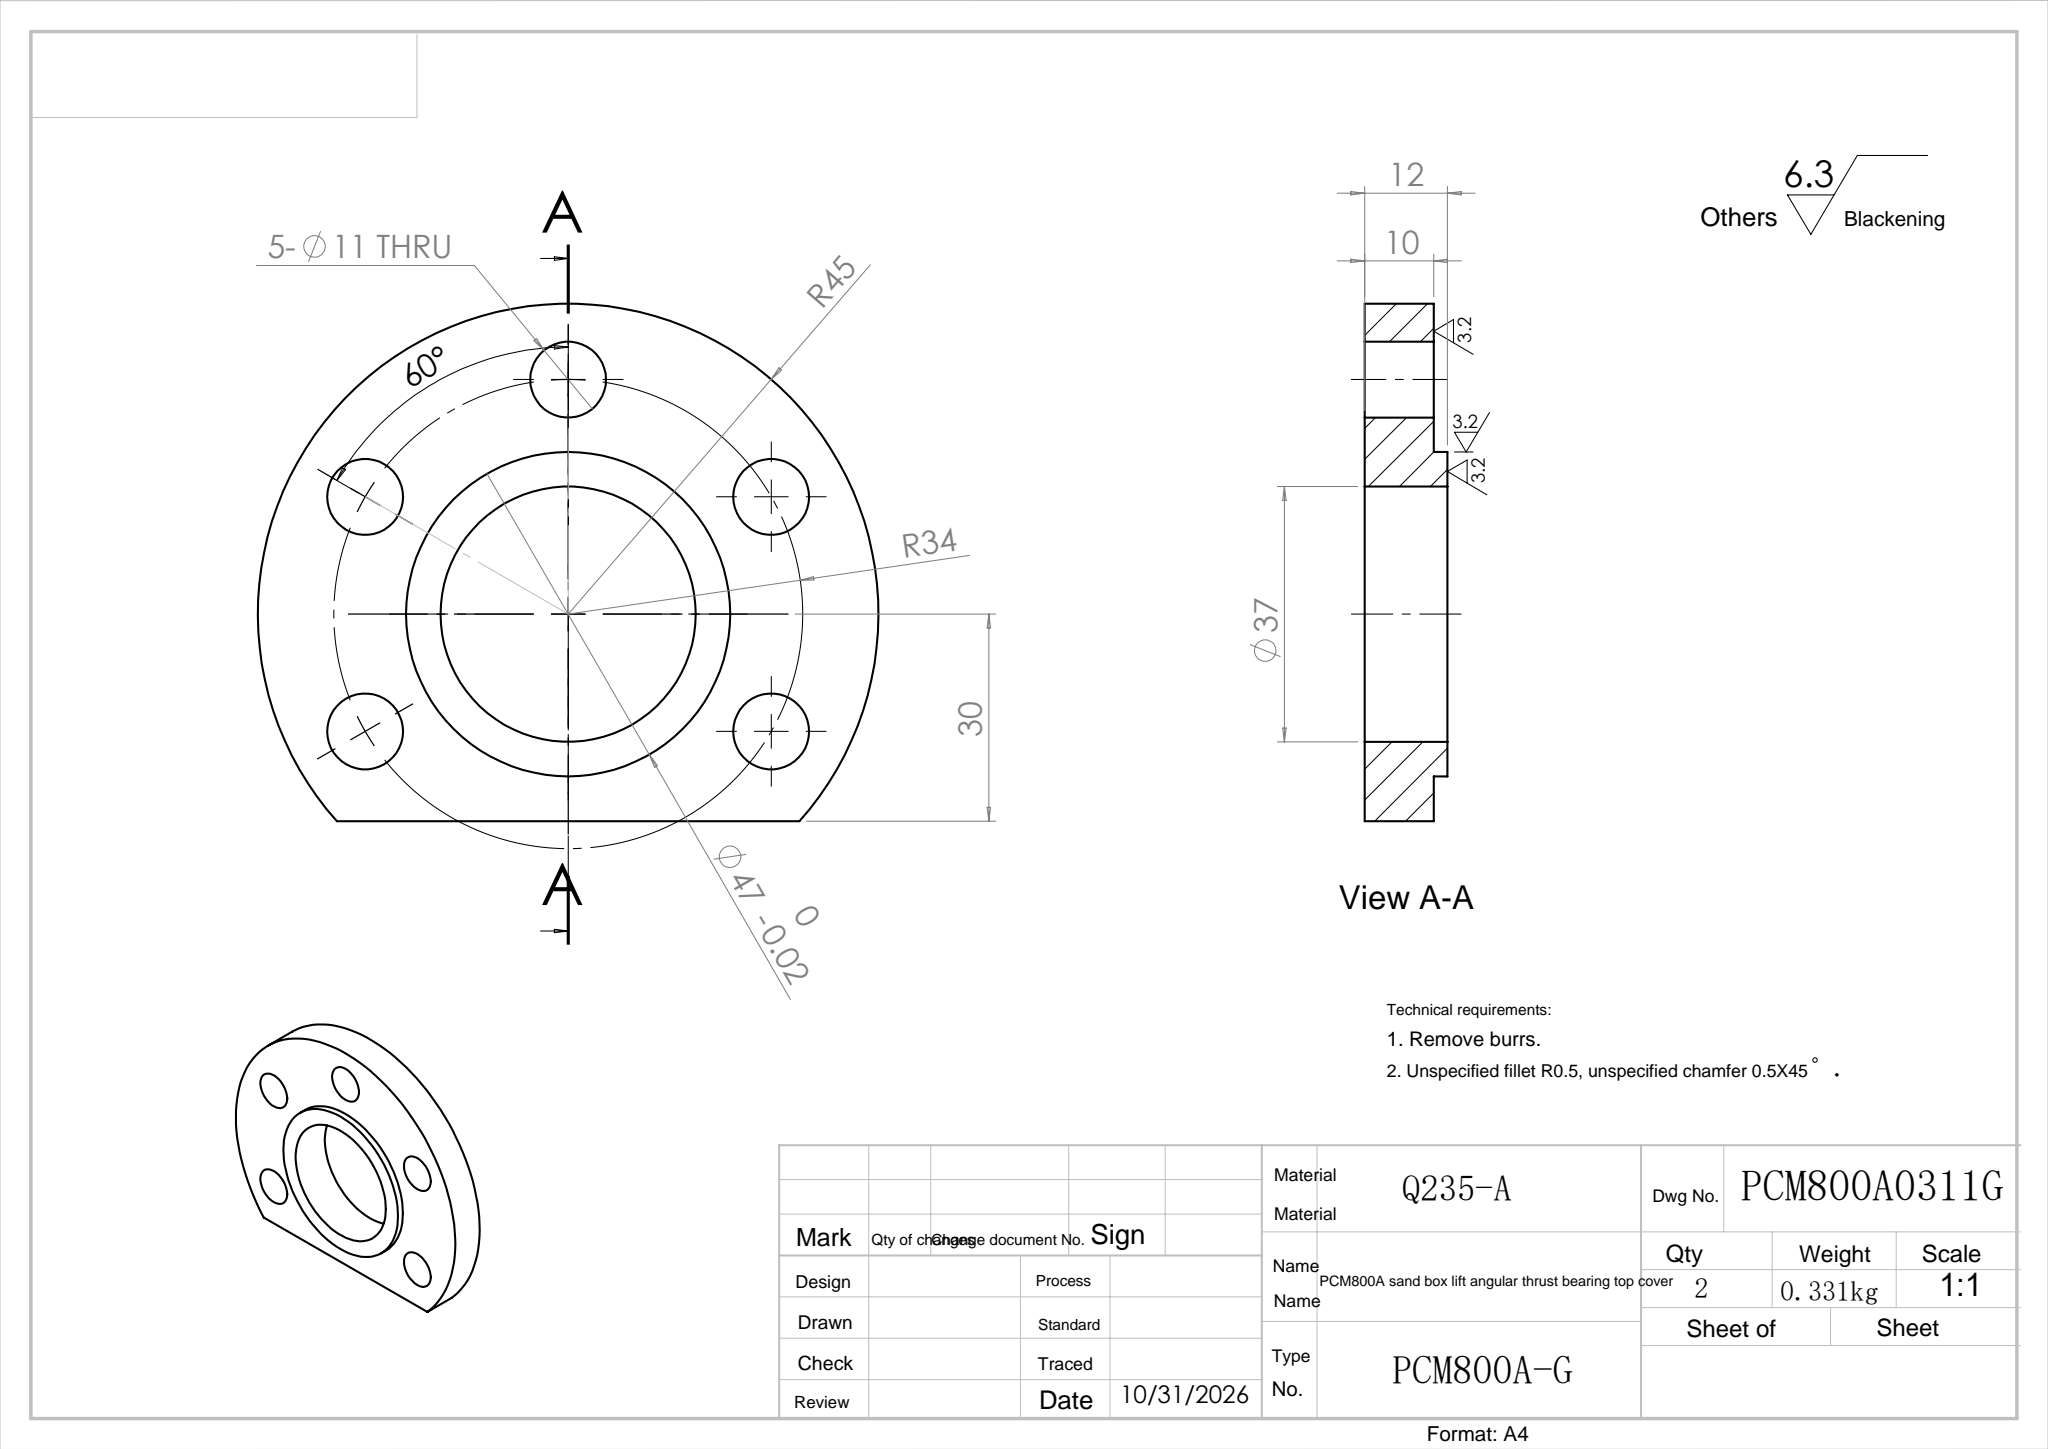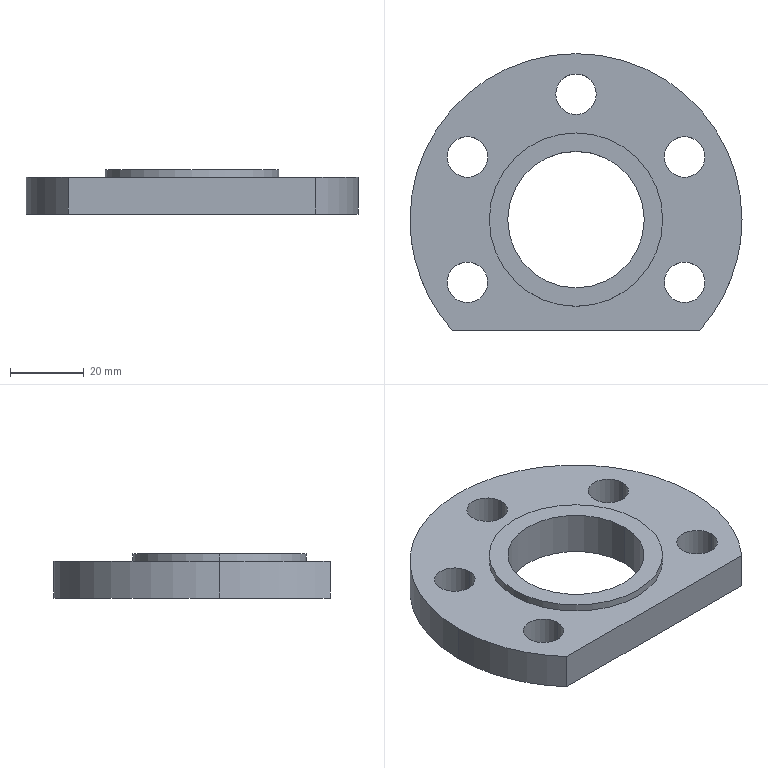Part | SolidWorks | features Cut 2, Boss 1, Extrusion 1 | 1 solid | 21 faces | box 90 x 75 x 12 mm | volume 42464 mm3 | cylinder 17 | plane 4 | commonest cylinder face diameters 11 x10 90 x3 37 x2 47 x2
STEP:
#1=CARTESIAN_POINT('',(23.945,-17.,0.));
#2=VERTEX_POINT('',#1);
#3=CARTESIAN_POINT('',(34.945,-17.,0.));
#4=VERTEX_POINT('',#3);
#5=CARTESIAN_POINT('',(29.445,-17.,0.));
#6=DIRECTION('',(0.,0.,1.));
#7=DIRECTION('',(1.,0.,0.));
#8=AXIS2_PLACEMENT_3D('',#5,#6,#7);
#9=CIRCLE('',#8,5.5);
#10=EDGE_CURVE('',#2,#4,#9,.T.);
#11=ORIENTED_EDGE('',*,*,#10,.F.);
#12=CARTESIAN_POINT('',(23.945,-17.,10.));
#13=VERTEX_POINT('',#12);
#14=CARTESIAN_POINT('',(23.945,-17.,0.));
#15=DIRECTION('',(0.,0.,1.));
#16=VECTOR('',#15,1000.);
#17=LINE('',#14,#16);
#18=EDGE_CURVE('',#2,#13,#17,.T.);
#19=ORIENTED_EDGE('',*,*,#18,.T.);
#20=CARTESIAN_POINT('',(34.945,-17.,10.));
#21=VERTEX_POINT('',#20);
#22=CARTESIAN_POINT('',(29.445,-17.,10.));
#23=DIRECTION('',(0.,0.,1.));
#24=DIRECTION('',(1.,0.,0.));
#25=AXIS2_PLACEMENT_3D('',#22,#23,#24);
#26=CIRCLE('',#25,5.5);
#27=EDGE_CURVE('',#13,#21,#26,.T.);
#28=ORIENTED_EDGE('',*,*,#27,.T.);
#29=CARTESIAN_POINT('',(34.945,-17.,0.));
#30=DIRECTION('',(0.,0.,1.));
#31=VECTOR('',#30,1000.);
#32=LINE('',#29,#31);
#33=EDGE_CURVE('',#4,#21,#32,.T.);
#34=ORIENTED_EDGE('',*,*,#33,.F.);
#35=EDGE_LOOP('',(#11,#19,#28,#34));
#36=FACE_OUTER_BOUND('',#35,.T.);
#37=CARTESIAN_POINT('',(29.445,-17.,0.));
#38=DIRECTION('',(0.,0.,1.));
#39=DIRECTION('',(1.,0.,0.));
#40=AXIS2_PLACEMENT_3D('',#37,#38,#39);
#41=CYLINDRICAL_SURFACE('',#40,5.5);
#42=ADVANCED_FACE('',(#36),#41,.F.);
#43=CARTESIAN_POINT('',(23.945,17.,0.));
#44=VERTEX_POINT('',#43);
#45=CARTESIAN_POINT('',(34.945,17.,0.));
#46=VERTEX_POINT('',#45);
#47=CARTESIAN_POINT('',(29.445,17.,0.));
#48=DIRECTION('',(0.,0.,1.));
#49=DIRECTION('',(1.,0.,0.));
#50=AXIS2_PLACEMENT_3D('',#47,#48,#49);
#51=CIRCLE('',#50,5.5);
#52=EDGE_CURVE('',#44,#46,#51,.T.);
#53=ORIENTED_EDGE('',*,*,#52,.F.);
#54=CARTESIAN_POINT('',(23.945,17.,10.));
#55=VERTEX_POINT('',#54);
#56=CARTESIAN_POINT('',(23.945,17.,0.));
#57=DIRECTION('',(0.,0.,1.));
#58=VECTOR('',#57,1000.);
#59=LINE('',#56,#58);
#60=EDGE_CURVE('',#44,#55,#59,.T.);
#61=ORIENTED_EDGE('',*,*,#60,.T.);
#62=CARTESIAN_POINT('',(34.945,17.,10.));
#63=VERTEX_POINT('',#62);
#64=CARTESIAN_POINT('',(29.445,17.,10.));
#65=DIRECTION('',(0.,0.,1.));
#66=DIRECTION('',(1.,0.,0.));
#67=AXIS2_PLACEMENT_3D('',#64,#65,#66);
#68=CIRCLE('',#67,5.5);
#69=EDGE_CURVE('',#55,#63,#68,.T.);
#70=ORIENTED_EDGE('',*,*,#69,.T.);
#71=CARTESIAN_POINT('',(34.945,17.,0.));
#72=DIRECTION('',(0.,0.,1.));
#73=VECTOR('',#72,1000.);
#74=LINE('',#71,#73);
#75=EDGE_CURVE('',#46,#63,#74,.T.);
#76=ORIENTED_EDGE('',*,*,#75,.F.);
#77=EDGE_LOOP('',(#53,#61,#70,#76));
#78=FACE_OUTER_BOUND('',#77,.T.);
#79=CARTESIAN_POINT('',(29.445,17.,0.));
#80=DIRECTION('',(0.,0.,1.));
#81=DIRECTION('',(1.,0.,0.));
#82=AXIS2_PLACEMENT_3D('',#79,#80,#81);
#83=CYLINDRICAL_SURFACE('',#82,5.5);
#84=ADVANCED_FACE('',(#78),#83,.F.);
#85=CARTESIAN_POINT('',(-34.945,-17.,0.));
#86=VERTEX_POINT('',#85);
#87=CARTESIAN_POINT('',(-23.945,-17.,0.));
#88=VERTEX_POINT('',#87);
#89=CARTESIAN_POINT('',(-29.445,-17.,0.));
#90=DIRECTION('',(0.,0.,1.));
#91=DIRECTION('',(1.,0.,0.));
#92=AXIS2_PLACEMENT_3D('',#89,#90,#91);
#93=CIRCLE('',#92,5.5);
#94=EDGE_CURVE('',#86,#88,#93,.T.);
#95=ORIENTED_EDGE('',*,*,#94,.F.);
#96=CARTESIAN_POINT('',(-34.945,-17.,10.));
#97=VERTEX_POINT('',#96);
#98=CARTESIAN_POINT('',(-34.945,-17.,0.));
#99=DIRECTION('',(0.,0.,1.));
#100=VECTOR('',#99,1000.);
#101=LINE('',#98,#100);
#102=EDGE_CURVE('',#86,#97,#101,.T.);
#103=ORIENTED_EDGE('',*,*,#102,.T.);
#104=CARTESIAN_POINT('',(-23.945,-17.,10.));
#105=VERTEX_POINT('',#104);
#106=CARTESIAN_POINT('',(-29.445,-17.,10.));
#107=DIRECTION('',(0.,0.,1.));
#108=DIRECTION('',(1.,0.,0.));
#109=AXIS2_PLACEMENT_3D('',#106,#107,#108);
#110=CIRCLE('',#109,5.5);
#111=EDGE_CURVE('',#97,#105,#110,.T.);
#112=ORIENTED_EDGE('',*,*,#111,.T.);
#113=CARTESIAN_POINT('',(-23.945,-17.,0.));
#114=DIRECTION('',(0.,0.,1.));
#115=VECTOR('',#114,1000.);
#116=LINE('',#113,#115);
#117=EDGE_CURVE('',#88,#105,#116,.T.);
#118=ORIENTED_EDGE('',*,*,#117,.F.);
#119=EDGE_LOOP('',(#95,#103,#112,#118));
#120=FACE_OUTER_BOUND('',#119,.T.);
#121=CARTESIAN_POINT('',(-29.445,-17.,0.));
#122=DIRECTION('',(0.,0.,1.));
#123=DIRECTION('',(1.,0.,0.));
#124=AXIS2_PLACEMENT_3D('',#121,#122,#123);
#125=CYLINDRICAL_SURFACE('',#124,5.5);
#126=ADVANCED_FACE('',(#120),#125,.F.);
#127=CARTESIAN_POINT('',(-34.945,17.,0.));
#128=VERTEX_POINT('',#127);
#129=CARTESIAN_POINT('',(-23.945,17.,0.));
#130=VERTEX_POINT('',#129);
#131=CARTESIAN_POINT('',(-29.445,17.,0.));
#132=DIRECTION('',(0.,0.,1.));
#133=DIRECTION('',(1.,0.,0.));
#134=AXIS2_PLACEMENT_3D('',#131,#132,#133);
#135=CIRCLE('',#134,5.5);
#136=EDGE_CURVE('',#128,#130,#135,.T.);
#137=ORIENTED_EDGE('',*,*,#136,.F.);
#138=CARTESIAN_POINT('',(-34.945,17.,10.));
#139=VERTEX_POINT('',#138);
#140=CARTESIAN_POINT('',(-34.945,17.,0.));
#141=DIRECTION('',(0.,0.,1.));
#142=VECTOR('',#141,1000.);
#143=LINE('',#140,#142);
#144=EDGE_CURVE('',#128,#139,#143,.T.);
#145=ORIENTED_EDGE('',*,*,#144,.T.);
#146=CARTESIAN_POINT('',(-23.945,17.,10.));
#147=VERTEX_POINT('',#146);
#148=CARTESIAN_POINT('',(-29.445,17.,10.));
#149=DIRECTION('',(0.,0.,1.));
#150=DIRECTION('',(1.,0.,0.));
#151=AXIS2_PLACEMENT_3D('',#148,#149,#150);
#152=CIRCLE('',#151,5.5);
#153=EDGE_CURVE('',#139,#147,#152,.T.);
#154=ORIENTED_EDGE('',*,*,#153,.T.);
#155=CARTESIAN_POINT('',(-23.945,17.,0.));
#156=DIRECTION('',(0.,0.,1.));
#157=VECTOR('',#156,1000.);
#158=LINE('',#155,#157);
#159=EDGE_CURVE('',#130,#147,#158,.T.);
#160=ORIENTED_EDGE('',*,*,#159,.F.);
#161=EDGE_LOOP('',(#137,#145,#154,#160));
#162=FACE_OUTER_BOUND('',#161,.T.);
#163=CARTESIAN_POINT('',(-29.445,17.,0.));
#164=DIRECTION('',(0.,0.,1.));
#165=DIRECTION('',(1.,0.,0.));
#166=AXIS2_PLACEMENT_3D('',#163,#164,#165);
#167=CYLINDRICAL_SURFACE('',#166,5.5);
#168=ADVANCED_FACE('',(#162),#167,.F.);
#169=CARTESIAN_POINT('',(-5.5,34.,0.));
#170=VERTEX_POINT('',#169);
#171=CARTESIAN_POINT('',(5.5,34.,0.));
#172=VERTEX_POINT('',#171);
#173=CARTESIAN_POINT('',(0.,34.,0.));
#174=DIRECTION('',(0.,0.,1.));
#175=DIRECTION('',(1.,0.,0.));
#176=AXIS2_PLACEMENT_3D('',#173,#174,#175);
#177=CIRCLE('',#176,5.5);
#178=EDGE_CURVE('',#170,#172,#177,.T.);
#179=ORIENTED_EDGE('',*,*,#178,.F.);
#180=CARTESIAN_POINT('',(-5.5,34.,10.));
#181=VERTEX_POINT('',#180);
#182=CARTESIAN_POINT('',(-5.5,34.,0.));
#183=DIRECTION('',(0.,0.,1.));
#184=VECTOR('',#183,1000.);
#185=LINE('',#182,#184);
#186=EDGE_CURVE('',#170,#181,#185,.T.);
#187=ORIENTED_EDGE('',*,*,#186,.T.);
#188=CARTESIAN_POINT('',(5.5,34.,10.));
#189=VERTEX_POINT('',#188);
#190=CARTESIAN_POINT('',(0.,34.,10.));
#191=DIRECTION('',(0.,0.,1.));
#192=DIRECTION('',(1.,0.,0.));
#193=AXIS2_PLACEMENT_3D('',#190,#191,#192);
#194=CIRCLE('',#193,5.5);
#195=EDGE_CURVE('',#181,#189,#194,.T.);
#196=ORIENTED_EDGE('',*,*,#195,.T.);
#197=CARTESIAN_POINT('',(5.5,34.,0.));
#198=DIRECTION('',(0.,0.,1.));
#199=VECTOR('',#198,1000.);
#200=LINE('',#197,#199);
#201=EDGE_CURVE('',#172,#189,#200,.T.);
#202=ORIENTED_EDGE('',*,*,#201,.F.);
#203=EDGE_LOOP('',(#179,#187,#196,#202));
#204=FACE_OUTER_BOUND('',#203,.T.);
#205=CARTESIAN_POINT('',(0.,34.,0.));
#206=DIRECTION('',(0.,0.,1.));
#207=DIRECTION('',(1.,0.,0.));
#208=AXIS2_PLACEMENT_3D('',#205,#206,#207);
#209=CYLINDRICAL_SURFACE('',#208,5.5);
#210=ADVANCED_FACE('',(#204),#209,.F.);
#211=CARTESIAN_POINT('',(23.5,0.,12.));
#212=VERTEX_POINT('',#211);
#213=CARTESIAN_POINT('',(-23.5,0.,12.));
#214=VERTEX_POINT('',#213);
#215=CARTESIAN_POINT('',(0.,0.,12.));
#216=DIRECTION('',(0.,0.,1.));
#217=DIRECTION('',(1.,0.,0.));
#218=AXIS2_PLACEMENT_3D('',#215,#216,#217);
#219=CIRCLE('',#218,23.5);
#220=EDGE_CURVE('',#212,#214,#219,.T.);
#221=ORIENTED_EDGE('',*,*,#220,.F.);
#222=CARTESIAN_POINT('',(23.5,0.,10.));
#223=VERTEX_POINT('',#222);
#224=CARTESIAN_POINT('',(23.5,0.,12.));
#225=DIRECTION('',(0.,0.,-1.));
#226=VECTOR('',#225,1000.);
#227=LINE('',#224,#226);
#228=EDGE_CURVE('',#212,#223,#227,.T.);
#229=ORIENTED_EDGE('',*,*,#228,.T.);
#230=CARTESIAN_POINT('',(-23.5,0.,10.));
#231=VERTEX_POINT('',#230);
#232=CARTESIAN_POINT('',(0.,0.,10.));
#233=DIRECTION('',(0.,0.,1.));
#234=DIRECTION('',(1.,0.,0.));
#235=AXIS2_PLACEMENT_3D('',#232,#233,#234);
#236=CIRCLE('',#235,23.5);
#237=EDGE_CURVE('',#223,#231,#236,.T.);
#238=ORIENTED_EDGE('',*,*,#237,.T.);
#239=CARTESIAN_POINT('',(-23.5,0.,12.));
#240=DIRECTION('',(0.,0.,-1.));
#241=VECTOR('',#240,1000.);
#242=LINE('',#239,#241);
#243=EDGE_CURVE('',#214,#231,#242,.T.);
#244=ORIENTED_EDGE('',*,*,#243,.F.);
#245=EDGE_LOOP('',(#221,#229,#238,#244));
#246=FACE_OUTER_BOUND('',#245,.T.);
#247=CARTESIAN_POINT('',(0.,0.,12.));
#248=DIRECTION('',(0.,0.,-1.));
#249=DIRECTION('',(-1.,0.,0.));
#250=AXIS2_PLACEMENT_3D('',#247,#248,#249);
#251=CYLINDRICAL_SURFACE('',#250,23.5);
#252=ADVANCED_FACE('',(#246),#251,.T.);
#253=CARTESIAN_POINT('',(-18.5,0.,12.));
#254=VERTEX_POINT('',#253);
#255=CARTESIAN_POINT('',(18.5,0.,12.));
#256=VERTEX_POINT('',#255);
#257=CARTESIAN_POINT('',(0.,0.,12.));
#258=DIRECTION('',(0.,0.,1.));
#259=DIRECTION('',(1.,0.,0.));
#260=AXIS2_PLACEMENT_3D('',#257,#258,#259);
#261=CIRCLE('',#260,18.5);
#262=EDGE_CURVE('',#254,#256,#261,.T.);
#263=ORIENTED_EDGE('',*,*,#262,.T.);
#264=CARTESIAN_POINT('',(18.5,0.,0.));
#265=VERTEX_POINT('',#264);
#266=CARTESIAN_POINT('',(18.5,0.,10.));
#267=DIRECTION('',(0.,0.,-1.));
#268=VECTOR('',#267,1000.);
#269=LINE('',#266,#268);
#270=EDGE_CURVE('',#256,#265,#269,.T.);
#271=ORIENTED_EDGE('',*,*,#270,.T.);
#272=CARTESIAN_POINT('',(-18.5,0.,0.));
#273=VERTEX_POINT('',#272);
#274=CARTESIAN_POINT('',(0.,0.,0.));
#275=DIRECTION('',(0.,0.,1.));
#276=DIRECTION('',(1.,0.,0.));
#277=AXIS2_PLACEMENT_3D('',#274,#275,#276);
#278=CIRCLE('',#277,18.5);
#279=EDGE_CURVE('',#273,#265,#278,.T.);
#280=ORIENTED_EDGE('',*,*,#279,.F.);
#281=CARTESIAN_POINT('',(-18.5,0.,10.));
#282=DIRECTION('',(0.,0.,-1.));
#283=VECTOR('',#282,1000.);
#284=LINE('',#281,#283);
#285=EDGE_CURVE('',#254,#273,#284,.T.);
#286=ORIENTED_EDGE('',*,*,#285,.F.);
#287=EDGE_LOOP('',(#263,#271,#280,#286));
#288=FACE_OUTER_BOUND('',#287,.T.);
#289=CARTESIAN_POINT('',(0.,0.,10.));
#290=DIRECTION('',(0.,0.,-1.));
#291=DIRECTION('',(-1.,0.,0.));
#292=AXIS2_PLACEMENT_3D('',#289,#290,#291);
#293=CYLINDRICAL_SURFACE('',#292,18.5);
#294=ADVANCED_FACE('',(#288),#293,.F.);
#295=CARTESIAN_POINT('',(45.,0.,10.));
#296=VERTEX_POINT('',#295);
#297=CARTESIAN_POINT('',(-45.,0.,10.));
#298=VERTEX_POINT('',#297);
#299=CARTESIAN_POINT('',(0.,0.,10.));
#300=DIRECTION('',(0.,0.,1.));
#301=DIRECTION('',(1.,0.,0.));
#302=AXIS2_PLACEMENT_3D('',#299,#300,#301);
#303=CIRCLE('',#302,45.);
#304=EDGE_CURVE('',#296,#298,#303,.T.);
#305=ORIENTED_EDGE('',*,*,#304,.F.);
#306=CARTESIAN_POINT('',(45.,0.,0.));
#307=VERTEX_POINT('',#306);
#308=CARTESIAN_POINT('',(45.,0.,10.));
#309=DIRECTION('',(0.,0.,-1.));
#310=VECTOR('',#309,1000.);
#311=LINE('',#308,#310);
#312=EDGE_CURVE('',#296,#307,#311,.T.);
#313=ORIENTED_EDGE('',*,*,#312,.T.);
#314=CARTESIAN_POINT('',(-45.,0.,0.));
#315=VERTEX_POINT('',#314);
#316=CARTESIAN_POINT('',(0.,0.,0.));
#317=DIRECTION('',(0.,0.,1.));
#318=DIRECTION('',(1.,0.,0.));
#319=AXIS2_PLACEMENT_3D('',#316,#317,#318);
#320=CIRCLE('',#319,45.);
#321=EDGE_CURVE('',#307,#315,#320,.T.);
#322=ORIENTED_EDGE('',*,*,#321,.T.);
#323=CARTESIAN_POINT('',(-45.,0.,10.));
#324=DIRECTION('',(0.,0.,-1.));
#325=VECTOR('',#324,1000.);
#326=LINE('',#323,#325);
#327=EDGE_CURVE('',#298,#315,#326,.T.);
#328=ORIENTED_EDGE('',*,*,#327,.F.);
#329=EDGE_LOOP('',(#305,#313,#322,#328));
#330=FACE_OUTER_BOUND('',#329,.T.);
#331=CARTESIAN_POINT('',(0.,0.,10.));
#332=DIRECTION('',(0.,0.,-1.));
#333=DIRECTION('',(-1.,0.,0.));
#334=AXIS2_PLACEMENT_3D('',#331,#332,#333);
#335=CYLINDRICAL_SURFACE('',#334,45.);
#336=ADVANCED_FACE('',(#330),#335,.T.);
#337=CARTESIAN_POINT('',(-33.541,-30.,10.));
#338=VERTEX_POINT('',#337);
#339=CARTESIAN_POINT('',(0.,0.,10.));
#340=DIRECTION('',(0.,0.,1.));
#341=DIRECTION('',(1.,0.,0.));
#342=AXIS2_PLACEMENT_3D('',#339,#340,#341);
#343=CIRCLE('',#342,45.);
#344=EDGE_CURVE('',#298,#338,#343,.T.);
#345=ORIENTED_EDGE('',*,*,#344,.F.);
#346=ORIENTED_EDGE('',*,*,#327,.T.);
#347=CARTESIAN_POINT('',(-33.541,-30.,0.));
#348=VERTEX_POINT('',#347);
#349=CARTESIAN_POINT('',(0.,0.,0.));
#350=DIRECTION('',(0.,0.,1.));
#351=DIRECTION('',(1.,0.,0.));
#352=AXIS2_PLACEMENT_3D('',#349,#350,#351);
#353=CIRCLE('',#352,45.);
#354=EDGE_CURVE('',#315,#348,#353,.T.);
#355=ORIENTED_EDGE('',*,*,#354,.T.);
#356=CARTESIAN_POINT('',(-33.541,-30.,10.));
#357=DIRECTION('',(0.,0.,1.));
#358=VECTOR('',#357,1000.);
#359=LINE('',#356,#358);
#360=EDGE_CURVE('',#348,#338,#359,.T.);
#361=ORIENTED_EDGE('',*,*,#360,.T.);
#362=EDGE_LOOP('',(#345,#346,#355,#361));
#363=FACE_OUTER_BOUND('',#362,.T.);
#364=CARTESIAN_POINT('',(0.,0.,10.));
#365=DIRECTION('',(0.,0.,-1.));
#366=DIRECTION('',(-1.,0.,0.));
#367=AXIS2_PLACEMENT_3D('',#364,#365,#366);
#368=CYLINDRICAL_SURFACE('',#367,45.);
#369=ADVANCED_FACE('',(#363),#368,.T.);
#370=CARTESIAN_POINT('',(33.541,-30.,10.));
#371=VERTEX_POINT('',#370);
#372=CARTESIAN_POINT('',(-35.389,-30.,10.));
#373=DIRECTION('',(-1.,0.,0.));
#374=VECTOR('',#373,1000.);
#375=LINE('',#372,#374);
#376=EDGE_CURVE('',#371,#338,#375,.T.);
#377=ORIENTED_EDGE('',*,*,#376,.F.);
#378=CARTESIAN_POINT('',(0.,0.,10.));
#379=DIRECTION('',(0.,0.,1.));
#380=DIRECTION('',(1.,0.,0.));
#381=AXIS2_PLACEMENT_3D('',#378,#379,#380);
#382=CIRCLE('',#381,45.);
#383=EDGE_CURVE('',#371,#296,#382,.T.);
#384=ORIENTED_EDGE('',*,*,#383,.T.);
#385=ORIENTED_EDGE('',*,*,#304,.T.);
#386=ORIENTED_EDGE('',*,*,#344,.T.);
#387=EDGE_LOOP('',(#377,#384,#385,#386));
#388=FACE_OUTER_BOUND('',#387,.T.);
#389=CARTESIAN_POINT('',(29.445,-17.,10.));
#390=DIRECTION('',(0.,0.,1.));
#391=DIRECTION('',(1.,0.,0.));
#392=AXIS2_PLACEMENT_3D('',#389,#390,#391);
#393=CIRCLE('',#392,5.5);
#394=EDGE_CURVE('',#21,#13,#393,.T.);
#395=ORIENTED_EDGE('',*,*,#394,.F.);
#396=ORIENTED_EDGE('',*,*,#27,.F.);
#397=EDGE_LOOP('',(#395,#396));
#398=FACE_BOUND('',#397,.T.);
#399=CARTESIAN_POINT('',(29.445,17.,10.));
#400=DIRECTION('',(0.,0.,1.));
#401=DIRECTION('',(1.,0.,0.));
#402=AXIS2_PLACEMENT_3D('',#399,#400,#401);
#403=CIRCLE('',#402,5.5);
#404=EDGE_CURVE('',#63,#55,#403,.T.);
#405=ORIENTED_EDGE('',*,*,#404,.F.);
#406=ORIENTED_EDGE('',*,*,#69,.F.);
#407=EDGE_LOOP('',(#405,#406));
#408=FACE_BOUND('',#407,.T.);
#409=CARTESIAN_POINT('',(-29.445,-17.,10.));
#410=DIRECTION('',(0.,0.,1.));
#411=DIRECTION('',(1.,0.,0.));
#412=AXIS2_PLACEMENT_3D('',#409,#410,#411);
#413=CIRCLE('',#412,5.5);
#414=EDGE_CURVE('',#105,#97,#413,.T.);
#415=ORIENTED_EDGE('',*,*,#414,.F.);
#416=ORIENTED_EDGE('',*,*,#111,.F.);
#417=EDGE_LOOP('',(#415,#416));
#418=FACE_BOUND('',#417,.T.);
#419=CARTESIAN_POINT('',(-29.445,17.,10.));
#420=DIRECTION('',(0.,0.,1.));
#421=DIRECTION('',(1.,0.,0.));
#422=AXIS2_PLACEMENT_3D('',#419,#420,#421);
#423=CIRCLE('',#422,5.5);
#424=EDGE_CURVE('',#147,#139,#423,.T.);
#425=ORIENTED_EDGE('',*,*,#424,.F.);
#426=ORIENTED_EDGE('',*,*,#153,.F.);
#427=EDGE_LOOP('',(#425,#426));
#428=FACE_BOUND('',#427,.T.);
#429=CARTESIAN_POINT('',(0.,34.,10.));
#430=DIRECTION('',(0.,0.,1.));
#431=DIRECTION('',(1.,0.,0.));
#432=AXIS2_PLACEMENT_3D('',#429,#430,#431);
#433=CIRCLE('',#432,5.5);
#434=EDGE_CURVE('',#189,#181,#433,.T.);
#435=ORIENTED_EDGE('',*,*,#434,.F.);
#436=ORIENTED_EDGE('',*,*,#195,.F.);
#437=EDGE_LOOP('',(#435,#436));
#438=FACE_BOUND('',#437,.T.);
#439=CARTESIAN_POINT('',(0.,0.,10.));
#440=DIRECTION('',(0.,0.,1.));
#441=DIRECTION('',(1.,0.,0.));
#442=AXIS2_PLACEMENT_3D('',#439,#440,#441);
#443=CIRCLE('',#442,23.5);
#444=EDGE_CURVE('',#231,#223,#443,.T.);
#445=ORIENTED_EDGE('',*,*,#444,.F.);
#446=ORIENTED_EDGE('',*,*,#237,.F.);
#447=EDGE_LOOP('',(#445,#446));
#448=FACE_BOUND('',#447,.T.);
#449=CARTESIAN_POINT('',(0.,0.,10.));
#450=DIRECTION('',(0.,0.,1.));
#451=DIRECTION('',(1.,0.,0.));
#452=AXIS2_PLACEMENT_3D('',#449,#450,#451);
#453=PLANE('',#452);
#454=ADVANCED_FACE('',(#388,#398,#408,#418,#428,#438,#448),#453,.T.);
#455=CARTESIAN_POINT('',(29.445,-17.,0.));
#456=DIRECTION('',(0.,0.,1.));
#457=DIRECTION('',(1.,0.,0.));
#458=AXIS2_PLACEMENT_3D('',#455,#456,#457);
#459=CIRCLE('',#458,5.5);
#460=EDGE_CURVE('',#4,#2,#459,.T.);
#461=ORIENTED_EDGE('',*,*,#460,.T.);
#462=ORIENTED_EDGE('',*,*,#10,.T.);
#463=EDGE_LOOP('',(#461,#462));
#464=FACE_BOUND('',#463,.T.);
#465=CARTESIAN_POINT('',(29.445,17.,0.));
#466=DIRECTION('',(0.,0.,1.));
#467=DIRECTION('',(1.,0.,0.));
#468=AXIS2_PLACEMENT_3D('',#465,#466,#467);
#469=CIRCLE('',#468,5.5);
#470=EDGE_CURVE('',#46,#44,#469,.T.);
#471=ORIENTED_EDGE('',*,*,#470,.T.);
#472=ORIENTED_EDGE('',*,*,#52,.T.);
#473=EDGE_LOOP('',(#471,#472));
#474=FACE_BOUND('',#473,.T.);
#475=CARTESIAN_POINT('',(-29.445,-17.,0.));
#476=DIRECTION('',(0.,0.,1.));
#477=DIRECTION('',(1.,0.,0.));
#478=AXIS2_PLACEMENT_3D('',#475,#476,#477);
#479=CIRCLE('',#478,5.5);
#480=EDGE_CURVE('',#88,#86,#479,.T.);
#481=ORIENTED_EDGE('',*,*,#480,.T.);
#482=ORIENTED_EDGE('',*,*,#94,.T.);
#483=EDGE_LOOP('',(#481,#482));
#484=FACE_BOUND('',#483,.T.);
#485=CARTESIAN_POINT('',(-29.445,17.,0.));
#486=DIRECTION('',(0.,0.,1.));
#487=DIRECTION('',(1.,0.,0.));
#488=AXIS2_PLACEMENT_3D('',#485,#486,#487);
#489=CIRCLE('',#488,5.5);
#490=EDGE_CURVE('',#130,#128,#489,.T.);
#491=ORIENTED_EDGE('',*,*,#490,.T.);
#492=ORIENTED_EDGE('',*,*,#136,.T.);
#493=EDGE_LOOP('',(#491,#492));
#494=FACE_BOUND('',#493,.T.);
#495=CARTESIAN_POINT('',(0.,34.,0.));
#496=DIRECTION('',(0.,0.,1.));
#497=DIRECTION('',(1.,0.,0.));
#498=AXIS2_PLACEMENT_3D('',#495,#496,#497);
#499=CIRCLE('',#498,5.5);
#500=EDGE_CURVE('',#172,#170,#499,.T.);
#501=ORIENTED_EDGE('',*,*,#500,.T.);
#502=ORIENTED_EDGE('',*,*,#178,.T.);
#503=EDGE_LOOP('',(#501,#502));
#504=FACE_BOUND('',#503,.T.);
#505=CARTESIAN_POINT('',(33.541,-30.,0.));
#506=VERTEX_POINT('',#505);
#507=CARTESIAN_POINT('',(0.,0.,0.));
#508=DIRECTION('',(0.,0.,1.));
#509=DIRECTION('',(1.,0.,0.));
#510=AXIS2_PLACEMENT_3D('',#507,#508,#509);
#511=CIRCLE('',#510,45.);
#512=EDGE_CURVE('',#506,#307,#511,.T.);
#513=ORIENTED_EDGE('',*,*,#512,.F.);
#514=CARTESIAN_POINT('',(-35.389,-30.,0.));
#515=DIRECTION('',(-1.,0.,0.));
#516=VECTOR('',#515,1000.);
#517=LINE('',#514,#516);
#518=EDGE_CURVE('',#506,#348,#517,.T.);
#519=ORIENTED_EDGE('',*,*,#518,.T.);
#520=ORIENTED_EDGE('',*,*,#354,.F.);
#521=ORIENTED_EDGE('',*,*,#321,.F.);
#522=EDGE_LOOP('',(#513,#519,#520,#521));
#523=FACE_OUTER_BOUND('',#522,.T.);
#524=ORIENTED_EDGE('',*,*,#279,.T.);
#525=CARTESIAN_POINT('',(0.,0.,0.));
#526=DIRECTION('',(0.,0.,1.));
#527=DIRECTION('',(1.,0.,0.));
#528=AXIS2_PLACEMENT_3D('',#525,#526,#527);
#529=CIRCLE('',#528,18.5);
#530=EDGE_CURVE('',#265,#273,#529,.T.);
#531=ORIENTED_EDGE('',*,*,#530,.T.);
#532=EDGE_LOOP('',(#524,#531));
#533=FACE_BOUND('',#532,.T.);
#534=CARTESIAN_POINT('',(0.,0.,0.));
#535=DIRECTION('',(0.,0.,1.));
#536=DIRECTION('',(1.,0.,0.));
#537=AXIS2_PLACEMENT_3D('',#534,#535,#536);
#538=PLANE('',#537);
#539=ADVANCED_FACE('',(#464,#474,#484,#494,#504,#523,#533),#538,.F.);
#540=ORIENTED_EDGE('',*,*,#312,.F.);
#541=ORIENTED_EDGE('',*,*,#383,.F.);
#542=CARTESIAN_POINT('',(33.541,-30.,10.));
#543=DIRECTION('',(0.,0.,-1.));
#544=VECTOR('',#543,1000.);
#545=LINE('',#542,#544);
#546=EDGE_CURVE('',#371,#506,#545,.T.);
#547=ORIENTED_EDGE('',*,*,#546,.T.);
#548=ORIENTED_EDGE('',*,*,#512,.T.);
#549=EDGE_LOOP('',(#540,#541,#547,#548));
#550=FACE_OUTER_BOUND('',#549,.T.);
#551=CARTESIAN_POINT('',(0.,0.,10.));
#552=DIRECTION('',(0.,0.,-1.));
#553=DIRECTION('',(-1.,0.,0.));
#554=AXIS2_PLACEMENT_3D('',#551,#552,#553);
#555=CYLINDRICAL_SURFACE('',#554,45.);
#556=ADVANCED_FACE('',(#550),#555,.T.);
#557=ORIENTED_EDGE('',*,*,#270,.F.);
#558=CARTESIAN_POINT('',(0.,0.,12.));
#559=DIRECTION('',(0.,0.,1.));
#560=DIRECTION('',(1.,0.,0.));
#561=AXIS2_PLACEMENT_3D('',#558,#559,#560);
#562=CIRCLE('',#561,18.5);
#563=EDGE_CURVE('',#256,#254,#562,.T.);
#564=ORIENTED_EDGE('',*,*,#563,.T.);
#565=ORIENTED_EDGE('',*,*,#285,.T.);
#566=ORIENTED_EDGE('',*,*,#530,.F.);
#567=EDGE_LOOP('',(#557,#564,#565,#566));
#568=FACE_OUTER_BOUND('',#567,.T.);
#569=CARTESIAN_POINT('',(0.,0.,10.));
#570=DIRECTION('',(0.,0.,-1.));
#571=DIRECTION('',(-1.,0.,0.));
#572=AXIS2_PLACEMENT_3D('',#569,#570,#571);
#573=CYLINDRICAL_SURFACE('',#572,18.5);
#574=ADVANCED_FACE('',(#568),#573,.F.);
#575=CARTESIAN_POINT('',(0.,0.,12.));
#576=DIRECTION('',(0.,0.,1.));
#577=DIRECTION('',(1.,0.,0.));
#578=AXIS2_PLACEMENT_3D('',#575,#576,#577);
#579=CIRCLE('',#578,23.5);
#580=EDGE_CURVE('',#214,#212,#579,.T.);
#581=ORIENTED_EDGE('',*,*,#580,.T.);
#582=ORIENTED_EDGE('',*,*,#220,.T.);
#583=EDGE_LOOP('',(#581,#582));
#584=FACE_OUTER_BOUND('',#583,.T.);
#585=ORIENTED_EDGE('',*,*,#262,.F.);
#586=ORIENTED_EDGE('',*,*,#563,.F.);
#587=EDGE_LOOP('',(#585,#586));
#588=FACE_BOUND('',#587,.T.);
#589=CARTESIAN_POINT('',(0.,0.,12.));
#590=DIRECTION('',(0.,0.,1.));
#591=DIRECTION('',(1.,0.,0.));
#592=AXIS2_PLACEMENT_3D('',#589,#590,#591);
#593=PLANE('',#592);
#594=ADVANCED_FACE('',(#584,#588),#593,.T.);
#595=ORIENTED_EDGE('',*,*,#228,.F.);
#596=ORIENTED_EDGE('',*,*,#580,.F.);
#597=ORIENTED_EDGE('',*,*,#243,.T.);
#598=ORIENTED_EDGE('',*,*,#444,.T.);
#599=EDGE_LOOP('',(#595,#596,#597,#598));
#600=FACE_OUTER_BOUND('',#599,.T.);
#601=CARTESIAN_POINT('',(0.,0.,12.));
#602=DIRECTION('',(0.,0.,-1.));
#603=DIRECTION('',(-1.,0.,0.));
#604=AXIS2_PLACEMENT_3D('',#601,#602,#603);
#605=CYLINDRICAL_SURFACE('',#604,23.5);
#606=ADVANCED_FACE('',(#600),#605,.T.);
#607=ORIENTED_EDGE('',*,*,#186,.F.);
#608=ORIENTED_EDGE('',*,*,#500,.F.);
#609=ORIENTED_EDGE('',*,*,#201,.T.);
#610=ORIENTED_EDGE('',*,*,#434,.T.);
#611=EDGE_LOOP('',(#607,#608,#609,#610));
#612=FACE_OUTER_BOUND('',#611,.T.);
#613=CARTESIAN_POINT('',(0.,34.,0.));
#614=DIRECTION('',(0.,0.,1.));
#615=DIRECTION('',(1.,0.,0.));
#616=AXIS2_PLACEMENT_3D('',#613,#614,#615);
#617=CYLINDRICAL_SURFACE('',#616,5.5);
#618=ADVANCED_FACE('',(#612),#617,.F.);
#619=ORIENTED_EDGE('',*,*,#144,.F.);
#620=ORIENTED_EDGE('',*,*,#490,.F.);
#621=ORIENTED_EDGE('',*,*,#159,.T.);
#622=ORIENTED_EDGE('',*,*,#424,.T.);
#623=EDGE_LOOP('',(#619,#620,#621,#622));
#624=FACE_OUTER_BOUND('',#623,.T.);
#625=CARTESIAN_POINT('',(-29.445,17.,0.));
#626=DIRECTION('',(0.,0.,1.));
#627=DIRECTION('',(1.,0.,0.));
#628=AXIS2_PLACEMENT_3D('',#625,#626,#627);
#629=CYLINDRICAL_SURFACE('',#628,5.5);
#630=ADVANCED_FACE('',(#624),#629,.F.);
#631=ORIENTED_EDGE('',*,*,#102,.F.);
#632=ORIENTED_EDGE('',*,*,#480,.F.);
#633=ORIENTED_EDGE('',*,*,#117,.T.);
#634=ORIENTED_EDGE('',*,*,#414,.T.);
#635=EDGE_LOOP('',(#631,#632,#633,#634));
#636=FACE_OUTER_BOUND('',#635,.T.);
#637=CARTESIAN_POINT('',(-29.445,-17.,0.));
#638=DIRECTION('',(0.,0.,1.));
#639=DIRECTION('',(1.,0.,0.));
#640=AXIS2_PLACEMENT_3D('',#637,#638,#639);
#641=CYLINDRICAL_SURFACE('',#640,5.5);
#642=ADVANCED_FACE('',(#636),#641,.F.);
#643=ORIENTED_EDGE('',*,*,#60,.F.);
#644=ORIENTED_EDGE('',*,*,#470,.F.);
#645=ORIENTED_EDGE('',*,*,#75,.T.);
#646=ORIENTED_EDGE('',*,*,#404,.T.);
#647=EDGE_LOOP('',(#643,#644,#645,#646));
#648=FACE_OUTER_BOUND('',#647,.T.);
#649=CARTESIAN_POINT('',(29.445,17.,0.));
#650=DIRECTION('',(0.,0.,1.));
#651=DIRECTION('',(1.,0.,0.));
#652=AXIS2_PLACEMENT_3D('',#649,#650,#651);
#653=CYLINDRICAL_SURFACE('',#652,5.5);
#654=ADVANCED_FACE('',(#648),#653,.F.);
#655=ORIENTED_EDGE('',*,*,#18,.F.);
#656=ORIENTED_EDGE('',*,*,#460,.F.);
#657=ORIENTED_EDGE('',*,*,#33,.T.);
#658=ORIENTED_EDGE('',*,*,#394,.T.);
#659=EDGE_LOOP('',(#655,#656,#657,#658));
#660=FACE_OUTER_BOUND('',#659,.T.);
#661=CARTESIAN_POINT('',(29.445,-17.,0.));
#662=DIRECTION('',(0.,0.,1.));
#663=DIRECTION('',(1.,0.,0.));
#664=AXIS2_PLACEMENT_3D('',#661,#662,#663);
#665=CYLINDRICAL_SURFACE('',#664,5.5);
#666=ADVANCED_FACE('',(#660),#665,.F.);
#667=ORIENTED_EDGE('',*,*,#376,.T.);
#668=ORIENTED_EDGE('',*,*,#360,.F.);
#669=ORIENTED_EDGE('',*,*,#518,.F.);
#670=ORIENTED_EDGE('',*,*,#546,.F.);
#671=EDGE_LOOP('',(#667,#668,#669,#670));
#672=FACE_OUTER_BOUND('',#671,.T.);
#673=CARTESIAN_POINT('',(-35.389,-30.,0.));
#674=DIRECTION('',(0.,1.,0.));
#675=DIRECTION('',(0.,0.,1.));
#676=AXIS2_PLACEMENT_3D('',#673,#674,#675);
#677=PLANE('',#676);
#678=ADVANCED_FACE('',(#672),#677,.F.);
#679=CLOSED_SHELL('',(#42,#84,#126,#168,#210,#252,#294,#336,#369,#454,#539,#556,#574,#594,#606,#618,#630,#642,#654,#666,#678));
#680=MANIFOLD_SOLID_BREP('',#679);
#681=CARTESIAN_POINT('',(0.,0.,0.));
#682=DIRECTION('',(0.,0.,1.));
#683=DIRECTION('',(1.,0.,0.));
#684=AXIS2_PLACEMENT_3D('',#681,#682,#683);
#685=(LENGTH_UNIT()NAMED_UNIT(*)SI_UNIT(.MILLI.,.METRE.));
#686=UNCERTAINTY_MEASURE_WITH_UNIT(LENGTH_MEASURE(0.00001),#685,'','');
#687=(NAMED_UNIT(*)PLANE_ANGLE_UNIT()SI_UNIT($,.RADIAN.));
#688=(NAMED_UNIT(*)SI_UNIT($,.STERADIAN.)SOLID_ANGLE_UNIT());
#689=(GEOMETRIC_REPRESENTATION_CONTEXT(3)GLOBAL_UNCERTAINTY_ASSIGNED_CONTEXT((#686))GLOBAL_UNIT_ASSIGNED_CONTEXT((#685,#687,#688))REPRESENTATION_CONTEXT('',''));
#690=ADVANCED_BREP_SHAPE_REPRESENTATION('',(#680,#684),#689);